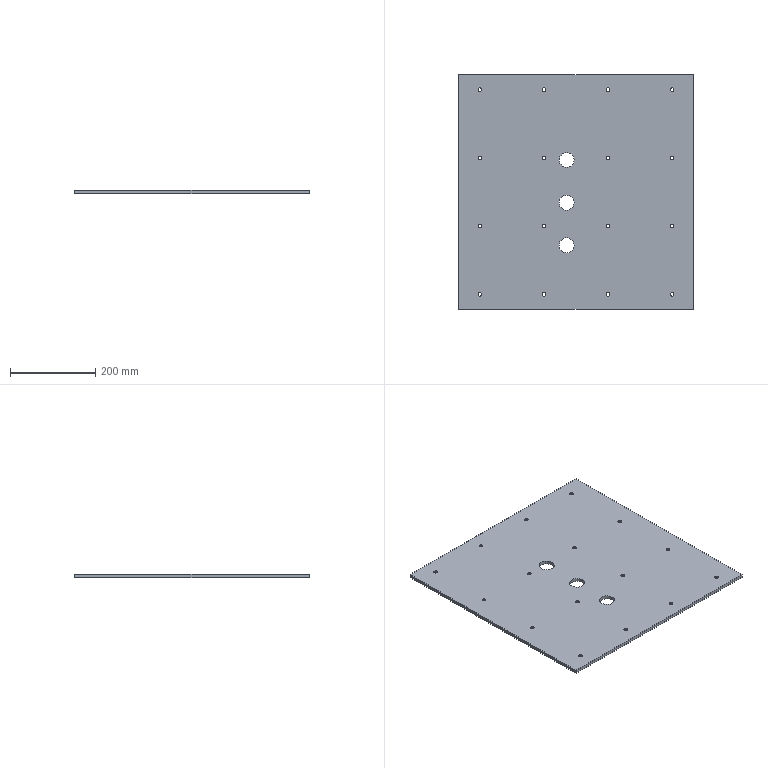Part | STEP file | 车灯-后视镜_id654_x_t | 1 solid | 57 faces | box 550 x 550 x 8 mm | volume 2381998 mm3 | cylinder 35 | cone 16 | plane 6 | commonest cylinder face diameters 8.5 x16 16 x16 35 x3
STEP:
#1=CARTESIAN_POINT('',(275.,-275.,-420.5));
#2=VERTEX_POINT('',#1);
#3=CARTESIAN_POINT('',(-275.,-275.,-420.5));
#4=VERTEX_POINT('',#3);
#5=CARTESIAN_POINT('',(275.,-275.,-420.5));
#6=DIRECTION('',(-1.,0.,0.));
#7=VECTOR('',#6,1.);
#8=LINE('',#5,#7);
#9=EDGE_CURVE('',#2,#4,#8,.T.);
#10=ORIENTED_EDGE('',*,*,#9,.T.);
#11=CARTESIAN_POINT('',(-275.,-275.,-428.5));
#12=VERTEX_POINT('',#11);
#13=CARTESIAN_POINT('',(-275.,-275.,-428.5));
#14=DIRECTION('',(0.,0.,1.));
#15=VECTOR('',#14,1.);
#16=LINE('',#13,#15);
#17=EDGE_CURVE('',#12,#4,#16,.T.);
#18=ORIENTED_EDGE('',*,*,#17,.F.);
#19=CARTESIAN_POINT('',(275.,-275.,-428.5));
#20=VERTEX_POINT('',#19);
#21=CARTESIAN_POINT('',(275.,-275.,-428.5));
#22=DIRECTION('',(-1.,0.,0.));
#23=VECTOR('',#22,1.);
#24=LINE('',#21,#23);
#25=EDGE_CURVE('',#20,#12,#24,.T.);
#26=ORIENTED_EDGE('',*,*,#25,.F.);
#27=CARTESIAN_POINT('',(275.,-275.,-428.5));
#28=DIRECTION('',(0.,0.,1.));
#29=VECTOR('',#28,1.);
#30=LINE('',#27,#29);
#31=EDGE_CURVE('',#20,#2,#30,.T.);
#32=ORIENTED_EDGE('',*,*,#31,.T.);
#33=EDGE_LOOP('',(#10,#18,#26,#32));
#34=FACE_OUTER_BOUND('',#33,.T.);
#35=CARTESIAN_POINT('',(275.,-275.,-428.5));
#36=DIRECTION('',(0.,-1.,0.));
#37=DIRECTION('',(0.,0.,1.));
#38=AXIS2_PLACEMENT_3D('',#35,#36,#37);
#39=PLANE('',#38);
#40=ADVANCED_FACE('',(#34),#39,.T.);
#41=CARTESIAN_POINT('',(-275.,275.,-420.5));
#42=VERTEX_POINT('',#41);
#43=CARTESIAN_POINT('',(-275.,-275.,-420.5));
#44=DIRECTION('',(0.,1.,0.));
#45=VECTOR('',#44,1.);
#46=LINE('',#43,#45);
#47=EDGE_CURVE('',#4,#42,#46,.T.);
#48=ORIENTED_EDGE('',*,*,#47,.T.);
#49=CARTESIAN_POINT('',(-275.,275.,-428.5));
#50=VERTEX_POINT('',#49);
#51=CARTESIAN_POINT('',(-275.,275.,-428.5));
#52=DIRECTION('',(0.,0.,1.));
#53=VECTOR('',#52,1.);
#54=LINE('',#51,#53);
#55=EDGE_CURVE('',#50,#42,#54,.T.);
#56=ORIENTED_EDGE('',*,*,#55,.F.);
#57=CARTESIAN_POINT('',(-275.,-275.,-428.5));
#58=DIRECTION('',(0.,1.,0.));
#59=VECTOR('',#58,1.);
#60=LINE('',#57,#59);
#61=EDGE_CURVE('',#12,#50,#60,.T.);
#62=ORIENTED_EDGE('',*,*,#61,.F.);
#63=ORIENTED_EDGE('',*,*,#17,.T.);
#64=EDGE_LOOP('',(#48,#56,#62,#63));
#65=FACE_OUTER_BOUND('',#64,.T.);
#66=CARTESIAN_POINT('',(-275.,-275.,-428.5));
#67=DIRECTION('',(-1.,0.,0.));
#68=DIRECTION('',(0.,0.,-1.));
#69=AXIS2_PLACEMENT_3D('',#66,#67,#68);
#70=PLANE('',#69);
#71=ADVANCED_FACE('',(#65),#70,.T.);
#72=CARTESIAN_POINT('',(275.,275.,-420.5));
#73=VERTEX_POINT('',#72);
#74=CARTESIAN_POINT('',(-275.,275.,-420.5));
#75=DIRECTION('',(1.,0.,0.));
#76=VECTOR('',#75,1.);
#77=LINE('',#74,#76);
#78=EDGE_CURVE('',#42,#73,#77,.T.);
#79=ORIENTED_EDGE('',*,*,#78,.T.);
#80=CARTESIAN_POINT('',(275.,275.,-428.5));
#81=VERTEX_POINT('',#80);
#82=CARTESIAN_POINT('',(275.,275.,-428.5));
#83=DIRECTION('',(0.,0.,1.));
#84=VECTOR('',#83,1.);
#85=LINE('',#82,#84);
#86=EDGE_CURVE('',#81,#73,#85,.T.);
#87=ORIENTED_EDGE('',*,*,#86,.F.);
#88=CARTESIAN_POINT('',(-275.,275.,-428.5));
#89=DIRECTION('',(1.,0.,0.));
#90=VECTOR('',#89,1.);
#91=LINE('',#88,#90);
#92=EDGE_CURVE('',#50,#81,#91,.T.);
#93=ORIENTED_EDGE('',*,*,#92,.F.);
#94=ORIENTED_EDGE('',*,*,#55,.T.);
#95=EDGE_LOOP('',(#79,#87,#93,#94));
#96=FACE_OUTER_BOUND('',#95,.T.);
#97=CARTESIAN_POINT('',(-275.,275.,-428.5));
#98=DIRECTION('',(0.,1.,0.));
#99=DIRECTION('',(0.,0.,-1.));
#100=AXIS2_PLACEMENT_3D('',#97,#98,#99);
#101=PLANE('',#100);
#102=ADVANCED_FACE('',(#96),#101,.T.);
#103=CARTESIAN_POINT('',(275.,275.,-420.5));
#104=DIRECTION('',(0.,-1.,0.));
#105=VECTOR('',#104,1.);
#106=LINE('',#103,#105);
#107=EDGE_CURVE('',#73,#2,#106,.T.);
#108=ORIENTED_EDGE('',*,*,#107,.T.);
#109=ORIENTED_EDGE('',*,*,#31,.F.);
#110=CARTESIAN_POINT('',(275.,275.,-428.5));
#111=DIRECTION('',(0.,-1.,0.));
#112=VECTOR('',#111,1.);
#113=LINE('',#110,#112);
#114=EDGE_CURVE('',#81,#20,#113,.T.);
#115=ORIENTED_EDGE('',*,*,#114,.F.);
#116=ORIENTED_EDGE('',*,*,#86,.T.);
#117=EDGE_LOOP('',(#108,#109,#115,#116));
#118=FACE_OUTER_BOUND('',#117,.T.);
#119=CARTESIAN_POINT('',(275.,275.,-428.5));
#120=DIRECTION('',(1.,0.,0.));
#121=DIRECTION('',(0.,0.,1.));
#122=AXIS2_PLACEMENT_3D('',#119,#120,#121);
#123=PLANE('',#122);
#124=ADVANCED_FACE('',(#118),#123,.T.);
#125=CARTESIAN_POINT('',(-83.,-80.,-428.5));
#126=VERTEX_POINT('',#125);
#127=CARTESIAN_POINT('',(-75.,-80.,-428.5));
#128=DIRECTION('',(0.,0.,-1.));
#129=DIRECTION('',(-1.,0.,0.));
#130=AXIS2_PLACEMENT_3D('',#127,#128,#129);
#131=CIRCLE('',#130,8.);
#132=EDGE_CURVE('',#126,#126,#131,.T.);
#133=ORIENTED_EDGE('',*,*,#132,.F.);
#134=EDGE_LOOP('',(#133));
#135=FACE_BOUND('',#134,.T.);
#136=CARTESIAN_POINT('',(-4.5,-125.,-428.5));
#137=VERTEX_POINT('',#136);
#138=CARTESIAN_POINT('',(-22.,-125.,-428.5));
#139=DIRECTION('',(0.,0.,1.));
#140=DIRECTION('',(1.,0.,0.));
#141=AXIS2_PLACEMENT_3D('',#138,#139,#140);
#142=CIRCLE('',#141,17.5);
#143=EDGE_CURVE('',#137,#137,#142,.T.);
#144=ORIENTED_EDGE('',*,*,#143,.T.);
#145=EDGE_LOOP('',(#144));
#146=FACE_BOUND('',#145,.T.);
#147=CARTESIAN_POINT('',(-4.5,-25.,-428.5));
#148=VERTEX_POINT('',#147);
#149=CARTESIAN_POINT('',(-22.,-25.,-428.5));
#150=DIRECTION('',(0.,0.,1.));
#151=DIRECTION('',(1.,0.,0.));
#152=AXIS2_PLACEMENT_3D('',#149,#150,#151);
#153=CIRCLE('',#152,17.5);
#154=EDGE_CURVE('',#148,#148,#153,.T.);
#155=ORIENTED_EDGE('',*,*,#154,.T.);
#156=EDGE_LOOP('',(#155));
#157=FACE_BOUND('',#156,.T.);
#158=CARTESIAN_POINT('',(-4.5,75.,-428.5));
#159=VERTEX_POINT('',#158);
#160=CARTESIAN_POINT('',(-22.,75.,-428.5));
#161=DIRECTION('',(0.,0.,1.));
#162=DIRECTION('',(1.,0.,0.));
#163=AXIS2_PLACEMENT_3D('',#160,#161,#162);
#164=CIRCLE('',#163,17.5);
#165=EDGE_CURVE('',#159,#159,#164,.T.);
#166=ORIENTED_EDGE('',*,*,#165,.T.);
#167=EDGE_LOOP('',(#166));
#168=FACE_BOUND('',#167,.T.);
#169=CARTESIAN_POINT('',(-233.,240.,-428.5));
#170=VERTEX_POINT('',#169);
#171=CARTESIAN_POINT('',(-225.,240.,-428.5));
#172=DIRECTION('',(0.,0.,-1.));
#173=DIRECTION('',(-1.,0.,0.));
#174=AXIS2_PLACEMENT_3D('',#171,#172,#173);
#175=CIRCLE('',#174,8.);
#176=EDGE_CURVE('',#170,#170,#175,.T.);
#177=ORIENTED_EDGE('',*,*,#176,.F.);
#178=EDGE_LOOP('',(#177));
#179=FACE_BOUND('',#178,.T.);
#180=CARTESIAN_POINT('',(-233.,-240.,-428.5));
#181=VERTEX_POINT('',#180);
#182=CARTESIAN_POINT('',(-225.,-240.,-428.5));
#183=DIRECTION('',(0.,0.,-1.));
#184=DIRECTION('',(-1.,0.,0.));
#185=AXIS2_PLACEMENT_3D('',#182,#183,#184);
#186=CIRCLE('',#185,8.);
#187=EDGE_CURVE('',#181,#181,#186,.T.);
#188=ORIENTED_EDGE('',*,*,#187,.F.);
#189=EDGE_LOOP('',(#188));
#190=FACE_BOUND('',#189,.T.);
#191=CARTESIAN_POINT('',(-83.,80.,-428.5));
#192=VERTEX_POINT('',#191);
#193=CARTESIAN_POINT('',(-75.,80.,-428.5));
#194=DIRECTION('',(0.,0.,-1.));
#195=DIRECTION('',(-1.,0.,0.));
#196=AXIS2_PLACEMENT_3D('',#193,#194,#195);
#197=CIRCLE('',#196,8.);
#198=EDGE_CURVE('',#192,#192,#197,.T.);
#199=ORIENTED_EDGE('',*,*,#198,.F.);
#200=EDGE_LOOP('',(#199));
#201=FACE_BOUND('',#200,.T.);
#202=CARTESIAN_POINT('',(-233.,-80.,-428.5));
#203=VERTEX_POINT('',#202);
#204=CARTESIAN_POINT('',(-225.,-80.,-428.5));
#205=DIRECTION('',(0.,0.,-1.));
#206=DIRECTION('',(-1.,0.,0.));
#207=AXIS2_PLACEMENT_3D('',#204,#205,#206);
#208=CIRCLE('',#207,8.);
#209=EDGE_CURVE('',#203,#203,#208,.T.);
#210=ORIENTED_EDGE('',*,*,#209,.F.);
#211=EDGE_LOOP('',(#210));
#212=FACE_BOUND('',#211,.T.);
#213=CARTESIAN_POINT('',(-233.,80.,-428.5));
#214=VERTEX_POINT('',#213);
#215=CARTESIAN_POINT('',(-225.,80.,-428.5));
#216=DIRECTION('',(0.,0.,-1.));
#217=DIRECTION('',(-1.,0.,0.));
#218=AXIS2_PLACEMENT_3D('',#215,#216,#217);
#219=CIRCLE('',#218,8.);
#220=EDGE_CURVE('',#214,#214,#219,.T.);
#221=ORIENTED_EDGE('',*,*,#220,.F.);
#222=EDGE_LOOP('',(#221));
#223=FACE_BOUND('',#222,.T.);
#224=CARTESIAN_POINT('',(-83.,-240.,-428.5));
#225=VERTEX_POINT('',#224);
#226=CARTESIAN_POINT('',(-75.,-240.,-428.5));
#227=DIRECTION('',(0.,0.,-1.));
#228=DIRECTION('',(-1.,0.,0.));
#229=AXIS2_PLACEMENT_3D('',#226,#227,#228);
#230=CIRCLE('',#229,8.);
#231=EDGE_CURVE('',#225,#225,#230,.T.);
#232=ORIENTED_EDGE('',*,*,#231,.F.);
#233=EDGE_LOOP('',(#232));
#234=FACE_BOUND('',#233,.T.);
#235=CARTESIAN_POINT('',(-83.,240.,-428.5));
#236=VERTEX_POINT('',#235);
#237=CARTESIAN_POINT('',(-75.,240.,-428.5));
#238=DIRECTION('',(0.,0.,-1.));
#239=DIRECTION('',(-1.,0.,0.));
#240=AXIS2_PLACEMENT_3D('',#237,#238,#239);
#241=CIRCLE('',#240,8.);
#242=EDGE_CURVE('',#236,#236,#241,.T.);
#243=ORIENTED_EDGE('',*,*,#242,.F.);
#244=EDGE_LOOP('',(#243));
#245=FACE_BOUND('',#244,.T.);
#246=CARTESIAN_POINT('',(67.,240.,-428.5));
#247=VERTEX_POINT('',#246);
#248=CARTESIAN_POINT('',(75.,240.,-428.5));
#249=DIRECTION('',(0.,0.,-1.));
#250=DIRECTION('',(-1.,0.,0.));
#251=AXIS2_PLACEMENT_3D('',#248,#249,#250);
#252=CIRCLE('',#251,8.);
#253=EDGE_CURVE('',#247,#247,#252,.T.);
#254=ORIENTED_EDGE('',*,*,#253,.F.);
#255=EDGE_LOOP('',(#254));
#256=FACE_BOUND('',#255,.T.);
#257=CARTESIAN_POINT('',(217.,80.,-428.5));
#258=VERTEX_POINT('',#257);
#259=CARTESIAN_POINT('',(225.,80.,-428.5));
#260=DIRECTION('',(0.,0.,-1.));
#261=DIRECTION('',(-1.,0.,0.));
#262=AXIS2_PLACEMENT_3D('',#259,#260,#261);
#263=CIRCLE('',#262,8.);
#264=EDGE_CURVE('',#258,#258,#263,.T.);
#265=ORIENTED_EDGE('',*,*,#264,.F.);
#266=EDGE_LOOP('',(#265));
#267=FACE_BOUND('',#266,.T.);
#268=CARTESIAN_POINT('',(217.,240.,-428.5));
#269=VERTEX_POINT('',#268);
#270=CARTESIAN_POINT('',(225.,240.,-428.5));
#271=DIRECTION('',(0.,0.,-1.));
#272=DIRECTION('',(-1.,0.,0.));
#273=AXIS2_PLACEMENT_3D('',#270,#271,#272);
#274=CIRCLE('',#273,8.);
#275=EDGE_CURVE('',#269,#269,#274,.T.);
#276=ORIENTED_EDGE('',*,*,#275,.F.);
#277=EDGE_LOOP('',(#276));
#278=FACE_BOUND('',#277,.T.);
#279=CARTESIAN_POINT('',(67.,-240.,-428.5));
#280=VERTEX_POINT('',#279);
#281=CARTESIAN_POINT('',(75.,-240.,-428.5));
#282=DIRECTION('',(0.,0.,-1.));
#283=DIRECTION('',(-1.,0.,0.));
#284=AXIS2_PLACEMENT_3D('',#281,#282,#283);
#285=CIRCLE('',#284,8.);
#286=EDGE_CURVE('',#280,#280,#285,.T.);
#287=ORIENTED_EDGE('',*,*,#286,.F.);
#288=EDGE_LOOP('',(#287));
#289=FACE_BOUND('',#288,.T.);
#290=CARTESIAN_POINT('',(217.,-240.,-428.5));
#291=VERTEX_POINT('',#290);
#292=CARTESIAN_POINT('',(225.,-240.,-428.5));
#293=DIRECTION('',(0.,0.,-1.));
#294=DIRECTION('',(-1.,0.,0.));
#295=AXIS2_PLACEMENT_3D('',#292,#293,#294);
#296=CIRCLE('',#295,8.);
#297=EDGE_CURVE('',#291,#291,#296,.T.);
#298=ORIENTED_EDGE('',*,*,#297,.F.);
#299=EDGE_LOOP('',(#298));
#300=FACE_BOUND('',#299,.T.);
#301=CARTESIAN_POINT('',(67.,-80.,-428.5));
#302=VERTEX_POINT('',#301);
#303=CARTESIAN_POINT('',(75.,-80.,-428.5));
#304=DIRECTION('',(0.,0.,-1.));
#305=DIRECTION('',(-1.,0.,0.));
#306=AXIS2_PLACEMENT_3D('',#303,#304,#305);
#307=CIRCLE('',#306,8.);
#308=EDGE_CURVE('',#302,#302,#307,.T.);
#309=ORIENTED_EDGE('',*,*,#308,.F.);
#310=EDGE_LOOP('',(#309));
#311=FACE_BOUND('',#310,.T.);
#312=CARTESIAN_POINT('',(217.,-80.,-428.5));
#313=VERTEX_POINT('',#312);
#314=CARTESIAN_POINT('',(225.,-80.,-428.5));
#315=DIRECTION('',(0.,0.,-1.));
#316=DIRECTION('',(-1.,0.,0.));
#317=AXIS2_PLACEMENT_3D('',#314,#315,#316);
#318=CIRCLE('',#317,8.);
#319=EDGE_CURVE('',#313,#313,#318,.T.);
#320=ORIENTED_EDGE('',*,*,#319,.F.);
#321=EDGE_LOOP('',(#320));
#322=FACE_BOUND('',#321,.T.);
#323=CARTESIAN_POINT('',(67.,80.,-428.5));
#324=VERTEX_POINT('',#323);
#325=CARTESIAN_POINT('',(75.,80.,-428.5));
#326=DIRECTION('',(0.,0.,-1.));
#327=DIRECTION('',(-1.,0.,0.));
#328=AXIS2_PLACEMENT_3D('',#325,#326,#327);
#329=CIRCLE('',#328,8.);
#330=EDGE_CURVE('',#324,#324,#329,.T.);
#331=ORIENTED_EDGE('',*,*,#330,.F.);
#332=EDGE_LOOP('',(#331));
#333=FACE_BOUND('',#332,.T.);
#334=ORIENTED_EDGE('',*,*,#25,.T.);
#335=ORIENTED_EDGE('',*,*,#61,.T.);
#336=ORIENTED_EDGE('',*,*,#92,.T.);
#337=ORIENTED_EDGE('',*,*,#114,.T.);
#338=EDGE_LOOP('',(#334,#335,#336,#337));
#339=FACE_BOUND('',#338,.T.);
#340=CARTESIAN_POINT('',(-275.,-275.,-428.5));
#341=DIRECTION('',(0.,0.,1.));
#342=DIRECTION('',(-1.,0.,0.));
#343=AXIS2_PLACEMENT_3D('',#340,#341,#342);
#344=PLANE('',#343);
#345=ADVANCED_FACE('',(#135,#146,#157,#168,#179,#190,#201,#212,#223,#234,#245,#256,#267,#278,#289,#300,#311,#322,#333,#339),#344,.F.);
#346=CARTESIAN_POINT('',(-79.25,-80.,-420.5));
#347=VERTEX_POINT('',#346);
#348=CARTESIAN_POINT('',(-75.,-80.,-420.5));
#349=DIRECTION('',(0.,0.,-1.));
#350=DIRECTION('',(-1.,0.,0.));
#351=AXIS2_PLACEMENT_3D('',#348,#349,#350);
#352=CIRCLE('',#351,4.25);
#353=EDGE_CURVE('',#347,#347,#352,.T.);
#354=ORIENTED_EDGE('',*,*,#353,.T.);
#355=EDGE_LOOP('',(#354));
#356=FACE_BOUND('',#355,.T.);
#357=CARTESIAN_POINT('',(-4.5,-125.,-420.5));
#358=VERTEX_POINT('',#357);
#359=CARTESIAN_POINT('',(-22.,-125.,-420.5));
#360=DIRECTION('',(0.,0.,1.));
#361=DIRECTION('',(1.,0.,0.));
#362=AXIS2_PLACEMENT_3D('',#359,#360,#361);
#363=CIRCLE('',#362,17.5);
#364=EDGE_CURVE('',#358,#358,#363,.T.);
#365=ORIENTED_EDGE('',*,*,#364,.F.);
#366=EDGE_LOOP('',(#365));
#367=FACE_BOUND('',#366,.T.);
#368=CARTESIAN_POINT('',(-4.5,-25.,-420.5));
#369=VERTEX_POINT('',#368);
#370=CARTESIAN_POINT('',(-22.,-25.,-420.5));
#371=DIRECTION('',(0.,0.,1.));
#372=DIRECTION('',(1.,0.,0.));
#373=AXIS2_PLACEMENT_3D('',#370,#371,#372);
#374=CIRCLE('',#373,17.5);
#375=EDGE_CURVE('',#369,#369,#374,.T.);
#376=ORIENTED_EDGE('',*,*,#375,.F.);
#377=EDGE_LOOP('',(#376));
#378=FACE_BOUND('',#377,.T.);
#379=CARTESIAN_POINT('',(-4.5,75.,-420.5));
#380=VERTEX_POINT('',#379);
#381=CARTESIAN_POINT('',(-22.,75.,-420.5));
#382=DIRECTION('',(0.,0.,1.));
#383=DIRECTION('',(1.,0.,0.));
#384=AXIS2_PLACEMENT_3D('',#381,#382,#383);
#385=CIRCLE('',#384,17.5);
#386=EDGE_CURVE('',#380,#380,#385,.T.);
#387=ORIENTED_EDGE('',*,*,#386,.F.);
#388=EDGE_LOOP('',(#387));
#389=FACE_BOUND('',#388,.T.);
#390=CARTESIAN_POINT('',(-229.25,240.,-420.5));
#391=VERTEX_POINT('',#390);
#392=CARTESIAN_POINT('',(-225.,240.,-420.5));
#393=DIRECTION('',(0.,0.,-1.));
#394=DIRECTION('',(-1.,0.,0.));
#395=AXIS2_PLACEMENT_3D('',#392,#393,#394);
#396=CIRCLE('',#395,4.25);
#397=EDGE_CURVE('',#391,#391,#396,.T.);
#398=ORIENTED_EDGE('',*,*,#397,.T.);
#399=EDGE_LOOP('',(#398));
#400=FACE_BOUND('',#399,.T.);
#401=CARTESIAN_POINT('',(-229.25,-240.,-420.5));
#402=VERTEX_POINT('',#401);
#403=CARTESIAN_POINT('',(-225.,-240.,-420.5));
#404=DIRECTION('',(0.,0.,-1.));
#405=DIRECTION('',(-1.,0.,0.));
#406=AXIS2_PLACEMENT_3D('',#403,#404,#405);
#407=CIRCLE('',#406,4.25);
#408=EDGE_CURVE('',#402,#402,#407,.T.);
#409=ORIENTED_EDGE('',*,*,#408,.T.);
#410=EDGE_LOOP('',(#409));
#411=FACE_BOUND('',#410,.T.);
#412=CARTESIAN_POINT('',(-79.25,80.,-420.5));
#413=VERTEX_POINT('',#412);
#414=CARTESIAN_POINT('',(-75.,80.,-420.5));
#415=DIRECTION('',(0.,0.,-1.));
#416=DIRECTION('',(-1.,0.,0.));
#417=AXIS2_PLACEMENT_3D('',#414,#415,#416);
#418=CIRCLE('',#417,4.25);
#419=EDGE_CURVE('',#413,#413,#418,.T.);
#420=ORIENTED_EDGE('',*,*,#419,.T.);
#421=EDGE_LOOP('',(#420));
#422=FACE_BOUND('',#421,.T.);
#423=CARTESIAN_POINT('',(-229.25,-80.,-420.5));
#424=VERTEX_POINT('',#423);
#425=CARTESIAN_POINT('',(-225.,-80.,-420.5));
#426=DIRECTION('',(0.,0.,-1.));
#427=DIRECTION('',(-1.,0.,0.));
#428=AXIS2_PLACEMENT_3D('',#425,#426,#427);
#429=CIRCLE('',#428,4.25);
#430=EDGE_CURVE('',#424,#424,#429,.T.);
#431=ORIENTED_EDGE('',*,*,#430,.T.);
#432=EDGE_LOOP('',(#431));
#433=FACE_BOUND('',#432,.T.);
#434=CARTESIAN_POINT('',(-229.25,80.,-420.5));
#435=VERTEX_POINT('',#434);
#436=CARTESIAN_POINT('',(-225.,80.,-420.5));
#437=DIRECTION('',(0.,0.,-1.));
#438=DIRECTION('',(-1.,0.,0.));
#439=AXIS2_PLACEMENT_3D('',#436,#437,#438);
#440=CIRCLE('',#439,4.25);
#441=EDGE_CURVE('',#435,#435,#440,.T.);
#442=ORIENTED_EDGE('',*,*,#441,.T.);
#443=EDGE_LOOP('',(#442));
#444=FACE_BOUND('',#443,.T.);
#445=CARTESIAN_POINT('',(-79.25,-240.,-420.5));
#446=VERTEX_POINT('',#445);
#447=CARTESIAN_POINT('',(-75.,-240.,-420.5));
#448=DIRECTION('',(0.,0.,-1.));
#449=DIRECTION('',(-1.,0.,0.));
#450=AXIS2_PLACEMENT_3D('',#447,#448,#449);
#451=CIRCLE('',#450,4.25);
#452=EDGE_CURVE('',#446,#446,#451,.T.);
#453=ORIENTED_EDGE('',*,*,#452,.T.);
#454=EDGE_LOOP('',(#453));
#455=FACE_BOUND('',#454,.T.);
#456=CARTESIAN_POINT('',(-79.25,240.,-420.5));
#457=VERTEX_POINT('',#456);
#458=CARTESIAN_POINT('',(-75.,240.,-420.5));
#459=DIRECTION('',(0.,0.,-1.));
#460=DIRECTION('',(-1.,0.,0.));
#461=AXIS2_PLACEMENT_3D('',#458,#459,#460);
#462=CIRCLE('',#461,4.25);
#463=EDGE_CURVE('',#457,#457,#462,.T.);
#464=ORIENTED_EDGE('',*,*,#463,.T.);
#465=EDGE_LOOP('',(#464));
#466=FACE_BOUND('',#465,.T.);
#467=CARTESIAN_POINT('',(70.75,240.,-420.5));
#468=VERTEX_POINT('',#467);
#469=CARTESIAN_POINT('',(75.,240.,-420.5));
#470=DIRECTION('',(0.,0.,-1.));
#471=DIRECTION('',(-1.,0.,0.));
#472=AXIS2_PLACEMENT_3D('',#469,#470,#471);
#473=CIRCLE('',#472,4.25);
#474=EDGE_CURVE('',#468,#468,#473,.T.);
#475=ORIENTED_EDGE('',*,*,#474,.T.);
#476=EDGE_LOOP('',(#475));
#477=FACE_BOUND('',#476,.T.);
#478=CARTESIAN_POINT('',(220.75,80.,-420.5));
#479=VERTEX_POINT('',#478);
#480=CARTESIAN_POINT('',(225.,80.,-420.5));
#481=DIRECTION('',(0.,0.,-1.));
#482=DIRECTION('',(-1.,0.,0.));
#483=AXIS2_PLACEMENT_3D('',#480,#481,#482);
#484=CIRCLE('',#483,4.25);
#485=EDGE_CURVE('',#479,#479,#484,.T.);
#486=ORIENTED_EDGE('',*,*,#485,.T.);
#487=EDGE_LOOP('',(#486));
#488=FACE_BOUND('',#487,.T.);
#489=CARTESIAN_POINT('',(220.75,240.,-420.5));
#490=VERTEX_POINT('',#489);
#491=CARTESIAN_POINT('',(225.,240.,-420.5));
#492=DIRECTION('',(0.,0.,-1.));
#493=DIRECTION('',(-1.,0.,0.));
#494=AXIS2_PLACEMENT_3D('',#491,#492,#493);
#495=CIRCLE('',#494,4.25);
#496=EDGE_CURVE('',#490,#490,#495,.T.);
#497=ORIENTED_EDGE('',*,*,#496,.T.);
#498=EDGE_LOOP('',(#497));
#499=FACE_BOUND('',#498,.T.);
#500=CARTESIAN_POINT('',(70.75,-240.,-420.5));
#501=VERTEX_POINT('',#500);
#502=CARTESIAN_POINT('',(75.,-240.,-420.5));
#503=DIRECTION('',(0.,0.,-1.));
#504=DIRECTION('',(-1.,0.,0.));
#505=AXIS2_PLACEMENT_3D('',#502,#503,#504);
#506=CIRCLE('',#505,4.25);
#507=EDGE_CURVE('',#501,#501,#506,.T.);
#508=ORIENTED_EDGE('',*,*,#507,.T.);
#509=EDGE_LOOP('',(#508));
#510=FACE_BOUND('',#509,.T.);
#511=CARTESIAN_POINT('',(220.75,-240.,-420.5));
#512=VERTEX_POINT('',#511);
#513=CARTESIAN_POINT('',(225.,-240.,-420.5));
#514=DIRECTION('',(0.,0.,-1.));
#515=DIRECTION('',(-1.,0.,0.));
#516=AXIS2_PLACEMENT_3D('',#513,#514,#515);
#517=CIRCLE('',#516,4.25);
#518=EDGE_CURVE('',#512,#512,#517,.T.);
#519=ORIENTED_EDGE('',*,*,#518,.T.);
#520=EDGE_LOOP('',(#519));
#521=FACE_BOUND('',#520,.T.);
#522=CARTESIAN_POINT('',(70.75,-80.,-420.5));
#523=VERTEX_POINT('',#522);
#524=CARTESIAN_POINT('',(75.,-80.,-420.5));
#525=DIRECTION('',(0.,0.,-1.));
#526=DIRECTION('',(-1.,0.,0.));
#527=AXIS2_PLACEMENT_3D('',#524,#525,#526);
#528=CIRCLE('',#527,4.25);
#529=EDGE_CURVE('',#523,#523,#528,.T.);
#530=ORIENTED_EDGE('',*,*,#529,.T.);
#531=EDGE_LOOP('',(#530));
#532=FACE_BOUND('',#531,.T.);
#533=CARTESIAN_POINT('',(220.75,-80.,-420.5));
#534=VERTEX_POINT('',#533);
#535=CARTESIAN_POINT('',(225.,-80.,-420.5));
#536=DIRECTION('',(0.,0.,-1.));
#537=DIRECTION('',(-1.,0.,0.));
#538=AXIS2_PLACEMENT_3D('',#535,#536,#537);
#539=CIRCLE('',#538,4.25);
#540=EDGE_CURVE('',#534,#534,#539,.T.);
#541=ORIENTED_EDGE('',*,*,#540,.T.);
#542=EDGE_LOOP('',(#541));
#543=FACE_BOUND('',#542,.T.);
#544=CARTESIAN_POINT('',(70.75,80.,-420.5));
#545=VERTEX_POINT('',#544);
#546=CARTESIAN_POINT('',(75.,80.,-420.5));
#547=DIRECTION('',(0.,0.,-1.));
#548=DIRECTION('',(-1.,0.,0.));
#549=AXIS2_PLACEMENT_3D('',#546,#547,#548);
#550=CIRCLE('',#549,4.25);
#551=EDGE_CURVE('',#545,#545,#550,.T.);
#552=ORIENTED_EDGE('',*,*,#551,.T.);
#553=EDGE_LOOP('',(#552));
#554=FACE_BOUND('',#553,.T.);
#555=ORIENTED_EDGE('',*,*,#9,.F.);
#556=ORIENTED_EDGE('',*,*,#107,.F.);
#557=ORIENTED_EDGE('',*,*,#78,.F.);
#558=ORIENTED_EDGE('',*,*,#47,.F.);
#559=EDGE_LOOP('',(#555,#556,#557,#558));
#560=FACE_BOUND('',#559,.T.);
#561=CARTESIAN_POINT('',(-275.,-275.,-420.5));
#562=DIRECTION('',(0.,0.,1.));
#563=DIRECTION('',(-1.,0.,0.));
#564=AXIS2_PLACEMENT_3D('',#561,#562,#563);
#565=PLANE('',#564);
#566=ADVANCED_FACE('',(#356,#367,#378,#389,#400,#411,#422,#433,#444,#455,#466,#477,#488,#499,#510,#521,#532,#543,#554,#560),#565,.T.);
#567=ORIENTED_EDGE('',*,*,#551,.F.);
#568=EDGE_LOOP('',(#567));
#569=FACE_BOUND('',#568,.T.);
#570=CARTESIAN_POINT('',(70.75,80.,-423.122));
#571=VERTEX_POINT('',#570);
#572=CARTESIAN_POINT('',(75.,80.,-423.122));
#573=DIRECTION('',(0.,0.,-1.));
#574=DIRECTION('',(-1.,0.,0.));
#575=AXIS2_PLACEMENT_3D('',#572,#573,#574);
#576=CIRCLE('',#575,4.25);
#577=EDGE_CURVE('',#571,#571,#576,.T.);
#578=ORIENTED_EDGE('',*,*,#577,.T.);
#579=EDGE_LOOP('',(#578));
#580=FACE_BOUND('',#579,.T.);
#581=CARTESIAN_POINT('',(75.,80.,-423.6));
#582=DIRECTION('',(0.,0.,1.));
#583=DIRECTION('',(1.,0.,0.));
#584=AXIS2_PLACEMENT_3D('',#581,#582,#583);
#585=CYLINDRICAL_SURFACE('',#584,4.25);
#586=ADVANCED_FACE('',(#569,#580),#585,.F.);
#587=CARTESIAN_POINT('',(67.,80.,-426.872));
#588=VERTEX_POINT('',#587);
#589=CARTESIAN_POINT('',(75.,80.,-426.872));
#590=DIRECTION('',(0.,0.,-1.));
#591=DIRECTION('',(-1.,0.,0.));
#592=AXIS2_PLACEMENT_3D('',#589,#590,#591);
#593=CIRCLE('',#592,8.);
#594=EDGE_CURVE('',#588,#588,#593,.T.);
#595=ORIENTED_EDGE('',*,*,#594,.F.);
#596=EDGE_LOOP('',(#595));
#597=FACE_BOUND('',#596,.T.);
#598=ORIENTED_EDGE('',*,*,#330,.T.);
#599=EDGE_LOOP('',(#598));
#600=FACE_BOUND('',#599,.T.);
#601=CARTESIAN_POINT('',(75.,80.,-428.));
#602=DIRECTION('',(0.,0.,1.));
#603=DIRECTION('',(1.,0.,0.));
#604=AXIS2_PLACEMENT_3D('',#601,#602,#603);
#605=CYLINDRICAL_SURFACE('',#604,8.);
#606=ADVANCED_FACE('',(#597,#600),#605,.F.);
#607=ORIENTED_EDGE('',*,*,#577,.F.);
#608=EDGE_LOOP('',(#607));
#609=FACE_BOUND('',#608,.T.);
#610=ORIENTED_EDGE('',*,*,#594,.T.);
#611=EDGE_LOOP('',(#610));
#612=FACE_BOUND('',#611,.T.);
#613=CARTESIAN_POINT('',(75.,80.,-426.286));
#614=DIRECTION('',(0.,0.,-1.));
#615=DIRECTION('',(1.,0.,0.));
#616=AXIS2_PLACEMENT_3D('',#613,#614,#615);
#617=CONICAL_SURFACE('',#616,7.414,45.);
#618=ADVANCED_FACE('',(#609,#612),#617,.F.);
#619=ORIENTED_EDGE('',*,*,#540,.F.);
#620=EDGE_LOOP('',(#619));
#621=FACE_BOUND('',#620,.T.);
#622=CARTESIAN_POINT('',(220.75,-80.,-423.122));
#623=VERTEX_POINT('',#622);
#624=CARTESIAN_POINT('',(225.,-80.,-423.122));
#625=DIRECTION('',(0.,0.,-1.));
#626=DIRECTION('',(-1.,0.,0.));
#627=AXIS2_PLACEMENT_3D('',#624,#625,#626);
#628=CIRCLE('',#627,4.25);
#629=EDGE_CURVE('',#623,#623,#628,.T.);
#630=ORIENTED_EDGE('',*,*,#629,.T.);
#631=EDGE_LOOP('',(#630));
#632=FACE_BOUND('',#631,.T.);
#633=CARTESIAN_POINT('',(225.,-80.,-423.6));
#634=DIRECTION('',(0.,0.,1.));
#635=DIRECTION('',(1.,0.,0.));
#636=AXIS2_PLACEMENT_3D('',#633,#634,#635);
#637=CYLINDRICAL_SURFACE('',#636,4.25);
#638=ADVANCED_FACE('',(#621,#632),#637,.F.);
#639=CARTESIAN_POINT('',(217.,-80.,-426.872));
#640=VERTEX_POINT('',#639);
#641=CARTESIAN_POINT('',(225.,-80.,-426.872));
#642=DIRECTION('',(0.,0.,-1.));
#643=DIRECTION('',(-1.,0.,0.));
#644=AXIS2_PLACEMENT_3D('',#641,#642,#643);
#645=CIRCLE('',#644,8.);
#646=EDGE_CURVE('',#640,#640,#645,.T.);
#647=ORIENTED_EDGE('',*,*,#646,.F.);
#648=EDGE_LOOP('',(#647));
#649=FACE_BOUND('',#648,.T.);
#650=ORIENTED_EDGE('',*,*,#319,.T.);
#651=EDGE_LOOP('',(#650));
#652=FACE_BOUND('',#651,.T.);
#653=CARTESIAN_POINT('',(225.,-80.,-428.));
#654=DIRECTION('',(0.,0.,1.));
#655=DIRECTION('',(1.,0.,0.));
#656=AXIS2_PLACEMENT_3D('',#653,#654,#655);
#657=CYLINDRICAL_SURFACE('',#656,8.);
#658=ADVANCED_FACE('',(#649,#652),#657,.F.);
#659=ORIENTED_EDGE('',*,*,#629,.F.);
#660=EDGE_LOOP('',(#659));
#661=FACE_BOUND('',#660,.T.);
#662=ORIENTED_EDGE('',*,*,#646,.T.);
#663=EDGE_LOOP('',(#662));
#664=FACE_BOUND('',#663,.T.);
#665=CARTESIAN_POINT('',(225.,-80.,-426.286));
#666=DIRECTION('',(0.,0.,-1.));
#667=DIRECTION('',(1.,0.,0.));
#668=AXIS2_PLACEMENT_3D('',#665,#666,#667);
#669=CONICAL_SURFACE('',#668,7.414,45.);
#670=ADVANCED_FACE('',(#661,#664),#669,.F.);
#671=ORIENTED_EDGE('',*,*,#529,.F.);
#672=EDGE_LOOP('',(#671));
#673=FACE_BOUND('',#672,.T.);
#674=CARTESIAN_POINT('',(70.75,-80.,-423.122));
#675=VERTEX_POINT('',#674);
#676=CARTESIAN_POINT('',(75.,-80.,-423.122));
#677=DIRECTION('',(0.,0.,-1.));
#678=DIRECTION('',(-1.,0.,0.));
#679=AXIS2_PLACEMENT_3D('',#676,#677,#678);
#680=CIRCLE('',#679,4.25);
#681=EDGE_CURVE('',#675,#675,#680,.T.);
#682=ORIENTED_EDGE('',*,*,#681,.T.);
#683=EDGE_LOOP('',(#682));
#684=FACE_BOUND('',#683,.T.);
#685=CARTESIAN_POINT('',(75.,-80.,-423.6));
#686=DIRECTION('',(0.,0.,1.));
#687=DIRECTION('',(1.,0.,0.));
#688=AXIS2_PLACEMENT_3D('',#685,#686,#687);
#689=CYLINDRICAL_SURFACE('',#688,4.25);
#690=ADVANCED_FACE('',(#673,#684),#689,.F.);
#691=CARTESIAN_POINT('',(67.,-80.,-426.872));
#692=VERTEX_POINT('',#691);
#693=CARTESIAN_POINT('',(75.,-80.,-426.872));
#694=DIRECTION('',(0.,0.,-1.));
#695=DIRECTION('',(-1.,0.,0.));
#696=AXIS2_PLACEMENT_3D('',#693,#694,#695);
#697=CIRCLE('',#696,8.);
#698=EDGE_CURVE('',#692,#692,#697,.T.);
#699=ORIENTED_EDGE('',*,*,#698,.F.);
#700=EDGE_LOOP('',(#699));
#701=FACE_BOUND('',#700,.T.);
#702=ORIENTED_EDGE('',*,*,#308,.T.);
#703=EDGE_LOOP('',(#702));
#704=FACE_BOUND('',#703,.T.);
#705=CARTESIAN_POINT('',(75.,-80.,-428.));
#706=DIRECTION('',(0.,0.,1.));
#707=DIRECTION('',(1.,0.,0.));
#708=AXIS2_PLACEMENT_3D('',#705,#706,#707);
#709=CYLINDRICAL_SURFACE('',#708,8.);
#710=ADVANCED_FACE('',(#701,#704),#709,.F.);
#711=ORIENTED_EDGE('',*,*,#681,.F.);
#712=EDGE_LOOP('',(#711));
#713=FACE_BOUND('',#712,.T.);
#714=ORIENTED_EDGE('',*,*,#698,.T.);
#715=EDGE_LOOP('',(#714));
#716=FACE_BOUND('',#715,.T.);
#717=CARTESIAN_POINT('',(75.,-80.,-426.286));
#718=DIRECTION('',(0.,0.,-1.));
#719=DIRECTION('',(1.,0.,0.));
#720=AXIS2_PLACEMENT_3D('',#717,#718,#719);
#721=CONICAL_SURFACE('',#720,7.414,45.);
#722=ADVANCED_FACE('',(#713,#716),#721,.F.);
#723=ORIENTED_EDGE('',*,*,#518,.F.);
#724=EDGE_LOOP('',(#723));
#725=FACE_BOUND('',#724,.T.);
#726=CARTESIAN_POINT('',(220.75,-240.,-423.122));
#727=VERTEX_POINT('',#726);
#728=CARTESIAN_POINT('',(225.,-240.,-423.122));
#729=DIRECTION('',(0.,0.,-1.));
#730=DIRECTION('',(-1.,0.,0.));
#731=AXIS2_PLACEMENT_3D('',#728,#729,#730);
#732=CIRCLE('',#731,4.25);
#733=EDGE_CURVE('',#727,#727,#732,.T.);
#734=ORIENTED_EDGE('',*,*,#733,.T.);
#735=EDGE_LOOP('',(#734));
#736=FACE_BOUND('',#735,.T.);
#737=CARTESIAN_POINT('',(225.,-240.,-423.6));
#738=DIRECTION('',(0.,0.,1.));
#739=DIRECTION('',(1.,0.,0.));
#740=AXIS2_PLACEMENT_3D('',#737,#738,#739);
#741=CYLINDRICAL_SURFACE('',#740,4.25);
#742=ADVANCED_FACE('',(#725,#736),#741,.F.);
#743=CARTESIAN_POINT('',(217.,-240.,-426.872));
#744=VERTEX_POINT('',#743);
#745=CARTESIAN_POINT('',(225.,-240.,-426.872));
#746=DIRECTION('',(0.,0.,-1.));
#747=DIRECTION('',(-1.,0.,0.));
#748=AXIS2_PLACEMENT_3D('',#745,#746,#747);
#749=CIRCLE('',#748,8.);
#750=EDGE_CURVE('',#744,#744,#749,.T.);
#751=ORIENTED_EDGE('',*,*,#750,.F.);
#752=EDGE_LOOP('',(#751));
#753=FACE_BOUND('',#752,.T.);
#754=ORIENTED_EDGE('',*,*,#297,.T.);
#755=EDGE_LOOP('',(#754));
#756=FACE_BOUND('',#755,.T.);
#757=CARTESIAN_POINT('',(225.,-240.,-428.));
#758=DIRECTION('',(0.,0.,1.));
#759=DIRECTION('',(1.,0.,0.));
#760=AXIS2_PLACEMENT_3D('',#757,#758,#759);
#761=CYLINDRICAL_SURFACE('',#760,8.);
#762=ADVANCED_FACE('',(#753,#756),#761,.F.);
#763=ORIENTED_EDGE('',*,*,#733,.F.);
#764=EDGE_LOOP('',(#763));
#765=FACE_BOUND('',#764,.T.);
#766=ORIENTED_EDGE('',*,*,#750,.T.);
#767=EDGE_LOOP('',(#766));
#768=FACE_BOUND('',#767,.T.);
#769=CARTESIAN_POINT('',(225.,-240.,-426.286));
#770=DIRECTION('',(0.,0.,-1.));
#771=DIRECTION('',(1.,0.,0.));
#772=AXIS2_PLACEMENT_3D('',#769,#770,#771);
#773=CONICAL_SURFACE('',#772,7.414,45.);
#774=ADVANCED_FACE('',(#765,#768),#773,.F.);
#775=ORIENTED_EDGE('',*,*,#507,.F.);
#776=EDGE_LOOP('',(#775));
#777=FACE_BOUND('',#776,.T.);
#778=CARTESIAN_POINT('',(70.75,-240.,-423.122));
#779=VERTEX_POINT('',#778);
#780=CARTESIAN_POINT('',(75.,-240.,-423.122));
#781=DIRECTION('',(0.,0.,-1.));
#782=DIRECTION('',(-1.,0.,0.));
#783=AXIS2_PLACEMENT_3D('',#780,#781,#782);
#784=CIRCLE('',#783,4.25);
#785=EDGE_CURVE('',#779,#779,#784,.T.);
#786=ORIENTED_EDGE('',*,*,#785,.T.);
#787=EDGE_LOOP('',(#786));
#788=FACE_BOUND('',#787,.T.);
#789=CARTESIAN_POINT('',(75.,-240.,-423.6));
#790=DIRECTION('',(0.,0.,1.));
#791=DIRECTION('',(1.,0.,0.));
#792=AXIS2_PLACEMENT_3D('',#789,#790,#791);
#793=CYLINDRICAL_SURFACE('',#792,4.25);
#794=ADVANCED_FACE('',(#777,#788),#793,.F.);
#795=CARTESIAN_POINT('',(67.,-240.,-426.872));
#796=VERTEX_POINT('',#795);
#797=CARTESIAN_POINT('',(75.,-240.,-426.872));
#798=DIRECTION('',(0.,0.,-1.));
#799=DIRECTION('',(-1.,0.,0.));
#800=AXIS2_PLACEMENT_3D('',#797,#798,#799);
#801=CIRCLE('',#800,8.);
#802=EDGE_CURVE('',#796,#796,#801,.T.);
#803=ORIENTED_EDGE('',*,*,#802,.F.);
#804=EDGE_LOOP('',(#803));
#805=FACE_BOUND('',#804,.T.);
#806=ORIENTED_EDGE('',*,*,#286,.T.);
#807=EDGE_LOOP('',(#806));
#808=FACE_BOUND('',#807,.T.);
#809=CARTESIAN_POINT('',(75.,-240.,-428.));
#810=DIRECTION('',(0.,0.,1.));
#811=DIRECTION('',(1.,0.,0.));
#812=AXIS2_PLACEMENT_3D('',#809,#810,#811);
#813=CYLINDRICAL_SURFACE('',#812,8.);
#814=ADVANCED_FACE('',(#805,#808),#813,.F.);
#815=ORIENTED_EDGE('',*,*,#785,.F.);
#816=EDGE_LOOP('',(#815));
#817=FACE_BOUND('',#816,.T.);
#818=ORIENTED_EDGE('',*,*,#802,.T.);
#819=EDGE_LOOP('',(#818));
#820=FACE_BOUND('',#819,.T.);
#821=CARTESIAN_POINT('',(75.,-240.,-426.286));
#822=DIRECTION('',(0.,0.,-1.));
#823=DIRECTION('',(1.,0.,0.));
#824=AXIS2_PLACEMENT_3D('',#821,#822,#823);
#825=CONICAL_SURFACE('',#824,7.414,45.);
#826=ADVANCED_FACE('',(#817,#820),#825,.F.);
#827=ORIENTED_EDGE('',*,*,#496,.F.);
#828=EDGE_LOOP('',(#827));
#829=FACE_BOUND('',#828,.T.);
#830=CARTESIAN_POINT('',(220.75,240.,-423.122));
#831=VERTEX_POINT('',#830);
#832=CARTESIAN_POINT('',(225.,240.,-423.122));
#833=DIRECTION('',(0.,0.,-1.));
#834=DIRECTION('',(-1.,0.,0.));
#835=AXIS2_PLACEMENT_3D('',#832,#833,#834);
#836=CIRCLE('',#835,4.25);
#837=EDGE_CURVE('',#831,#831,#836,.T.);
#838=ORIENTED_EDGE('',*,*,#837,.T.);
#839=EDGE_LOOP('',(#838));
#840=FACE_BOUND('',#839,.T.);
#841=CARTESIAN_POINT('',(225.,240.,-423.6));
#842=DIRECTION('',(0.,0.,1.));
#843=DIRECTION('',(1.,0.,0.));
#844=AXIS2_PLACEMENT_3D('',#841,#842,#843);
#845=CYLINDRICAL_SURFACE('',#844,4.25);
#846=ADVANCED_FACE('',(#829,#840),#845,.F.);
#847=CARTESIAN_POINT('',(217.,240.,-426.872));
#848=VERTEX_POINT('',#847);
#849=CARTESIAN_POINT('',(225.,240.,-426.872));
#850=DIRECTION('',(0.,0.,-1.));
#851=DIRECTION('',(-1.,0.,0.));
#852=AXIS2_PLACEMENT_3D('',#849,#850,#851);
#853=CIRCLE('',#852,8.);
#854=EDGE_CURVE('',#848,#848,#853,.T.);
#855=ORIENTED_EDGE('',*,*,#854,.F.);
#856=EDGE_LOOP('',(#855));
#857=FACE_BOUND('',#856,.T.);
#858=ORIENTED_EDGE('',*,*,#275,.T.);
#859=EDGE_LOOP('',(#858));
#860=FACE_BOUND('',#859,.T.);
#861=CARTESIAN_POINT('',(225.,240.,-428.));
#862=DIRECTION('',(0.,0.,1.));
#863=DIRECTION('',(1.,0.,0.));
#864=AXIS2_PLACEMENT_3D('',#861,#862,#863);
#865=CYLINDRICAL_SURFACE('',#864,8.);
#866=ADVANCED_FACE('',(#857,#860),#865,.F.);
#867=ORIENTED_EDGE('',*,*,#837,.F.);
#868=EDGE_LOOP('',(#867));
#869=FACE_BOUND('',#868,.T.);
#870=ORIENTED_EDGE('',*,*,#854,.T.);
#871=EDGE_LOOP('',(#870));
#872=FACE_BOUND('',#871,.T.);
#873=CARTESIAN_POINT('',(225.,240.,-426.286));
#874=DIRECTION('',(0.,0.,-1.));
#875=DIRECTION('',(1.,0.,0.));
#876=AXIS2_PLACEMENT_3D('',#873,#874,#875);
#877=CONICAL_SURFACE('',#876,7.414,45.);
#878=ADVANCED_FACE('',(#869,#872),#877,.F.);
#879=ORIENTED_EDGE('',*,*,#485,.F.);
#880=EDGE_LOOP('',(#879));
#881=FACE_BOUND('',#880,.T.);
#882=CARTESIAN_POINT('',(220.75,80.,-423.122));
#883=VERTEX_POINT('',#882);
#884=CARTESIAN_POINT('',(225.,80.,-423.122));
#885=DIRECTION('',(0.,0.,-1.));
#886=DIRECTION('',(-1.,0.,0.));
#887=AXIS2_PLACEMENT_3D('',#884,#885,#886);
#888=CIRCLE('',#887,4.25);
#889=EDGE_CURVE('',#883,#883,#888,.T.);
#890=ORIENTED_EDGE('',*,*,#889,.T.);
#891=EDGE_LOOP('',(#890));
#892=FACE_BOUND('',#891,.T.);
#893=CARTESIAN_POINT('',(225.,80.,-423.6));
#894=DIRECTION('',(0.,0.,1.));
#895=DIRECTION('',(1.,0.,0.));
#896=AXIS2_PLACEMENT_3D('',#893,#894,#895);
#897=CYLINDRICAL_SURFACE('',#896,4.25);
#898=ADVANCED_FACE('',(#881,#892),#897,.F.);
#899=CARTESIAN_POINT('',(217.,80.,-426.872));
#900=VERTEX_POINT('',#899);
#901=CARTESIAN_POINT('',(225.,80.,-426.872));
#902=DIRECTION('',(0.,0.,-1.));
#903=DIRECTION('',(-1.,0.,0.));
#904=AXIS2_PLACEMENT_3D('',#901,#902,#903);
#905=CIRCLE('',#904,8.);
#906=EDGE_CURVE('',#900,#900,#905,.T.);
#907=ORIENTED_EDGE('',*,*,#906,.F.);
#908=EDGE_LOOP('',(#907));
#909=FACE_BOUND('',#908,.T.);
#910=ORIENTED_EDGE('',*,*,#264,.T.);
#911=EDGE_LOOP('',(#910));
#912=FACE_BOUND('',#911,.T.);
#913=CARTESIAN_POINT('',(225.,80.,-428.));
#914=DIRECTION('',(0.,0.,1.));
#915=DIRECTION('',(1.,0.,0.));
#916=AXIS2_PLACEMENT_3D('',#913,#914,#915);
#917=CYLINDRICAL_SURFACE('',#916,8.);
#918=ADVANCED_FACE('',(#909,#912),#917,.F.);
#919=ORIENTED_EDGE('',*,*,#889,.F.);
#920=EDGE_LOOP('',(#919));
#921=FACE_BOUND('',#920,.T.);
#922=ORIENTED_EDGE('',*,*,#906,.T.);
#923=EDGE_LOOP('',(#922));
#924=FACE_BOUND('',#923,.T.);
#925=CARTESIAN_POINT('',(225.,80.,-426.286));
#926=DIRECTION('',(0.,0.,-1.));
#927=DIRECTION('',(1.,0.,0.));
#928=AXIS2_PLACEMENT_3D('',#925,#926,#927);
#929=CONICAL_SURFACE('',#928,7.414,45.);
#930=ADVANCED_FACE('',(#921,#924),#929,.F.);
#931=ORIENTED_EDGE('',*,*,#474,.F.);
#932=EDGE_LOOP('',(#931));
#933=FACE_BOUND('',#932,.T.);
#934=CARTESIAN_POINT('',(70.75,240.,-423.122));
#935=VERTEX_POINT('',#934);
#936=CARTESIAN_POINT('',(75.,240.,-423.122));
#937=DIRECTION('',(0.,0.,-1.));
#938=DIRECTION('',(-1.,0.,0.));
#939=AXIS2_PLACEMENT_3D('',#936,#937,#938);
#940=CIRCLE('',#939,4.25);
#941=EDGE_CURVE('',#935,#935,#940,.T.);
#942=ORIENTED_EDGE('',*,*,#941,.T.);
#943=EDGE_LOOP('',(#942));
#944=FACE_BOUND('',#943,.T.);
#945=CARTESIAN_POINT('',(75.,240.,-423.6));
#946=DIRECTION('',(0.,0.,1.));
#947=DIRECTION('',(1.,0.,0.));
#948=AXIS2_PLACEMENT_3D('',#945,#946,#947);
#949=CYLINDRICAL_SURFACE('',#948,4.25);
#950=ADVANCED_FACE('',(#933,#944),#949,.F.);
#951=CARTESIAN_POINT('',(67.,240.,-426.872));
#952=VERTEX_POINT('',#951);
#953=CARTESIAN_POINT('',(75.,240.,-426.872));
#954=DIRECTION('',(0.,0.,-1.));
#955=DIRECTION('',(-1.,0.,0.));
#956=AXIS2_PLACEMENT_3D('',#953,#954,#955);
#957=CIRCLE('',#956,8.);
#958=EDGE_CURVE('',#952,#952,#957,.T.);
#959=ORIENTED_EDGE('',*,*,#958,.F.);
#960=EDGE_LOOP('',(#959));
#961=FACE_BOUND('',#960,.T.);
#962=ORIENTED_EDGE('',*,*,#253,.T.);
#963=EDGE_LOOP('',(#962));
#964=FACE_BOUND('',#963,.T.);
#965=CARTESIAN_POINT('',(75.,240.,-428.));
#966=DIRECTION('',(0.,0.,1.));
#967=DIRECTION('',(1.,0.,0.));
#968=AXIS2_PLACEMENT_3D('',#965,#966,#967);
#969=CYLINDRICAL_SURFACE('',#968,8.);
#970=ADVANCED_FACE('',(#961,#964),#969,.F.);
#971=ORIENTED_EDGE('',*,*,#941,.F.);
#972=EDGE_LOOP('',(#971));
#973=FACE_BOUND('',#972,.T.);
#974=ORIENTED_EDGE('',*,*,#958,.T.);
#975=EDGE_LOOP('',(#974));
#976=FACE_BOUND('',#975,.T.);
#977=CARTESIAN_POINT('',(75.,240.,-426.286));
#978=DIRECTION('',(0.,0.,-1.));
#979=DIRECTION('',(1.,0.,0.));
#980=AXIS2_PLACEMENT_3D('',#977,#978,#979);
#981=CONICAL_SURFACE('',#980,7.414,45.);
#982=ADVANCED_FACE('',(#973,#976),#981,.F.);
#983=ORIENTED_EDGE('',*,*,#463,.F.);
#984=EDGE_LOOP('',(#983));
#985=FACE_BOUND('',#984,.T.);
#986=CARTESIAN_POINT('',(-79.25,240.,-423.122));
#987=VERTEX_POINT('',#986);
#988=CARTESIAN_POINT('',(-75.,240.,-423.122));
#989=DIRECTION('',(0.,0.,-1.));
#990=DIRECTION('',(-1.,0.,0.));
#991=AXIS2_PLACEMENT_3D('',#988,#989,#990);
#992=CIRCLE('',#991,4.25);
#993=EDGE_CURVE('',#987,#987,#992,.T.);
#994=ORIENTED_EDGE('',*,*,#993,.T.);
#995=EDGE_LOOP('',(#994));
#996=FACE_BOUND('',#995,.T.);
#997=CARTESIAN_POINT('',(-75.,240.,-423.6));
#998=DIRECTION('',(0.,0.,1.));
#999=DIRECTION('',(1.,0.,0.));
#1000=AXIS2_PLACEMENT_3D('',#997,#998,#999);
#1001=CYLINDRICAL_SURFACE('',#1000,4.25);
#1002=ADVANCED_FACE('',(#985,#996),#1001,.F.);
#1003=CARTESIAN_POINT('',(-83.,240.,-426.872));
#1004=VERTEX_POINT('',#1003);
#1005=CARTESIAN_POINT('',(-75.,240.,-426.872));
#1006=DIRECTION('',(0.,0.,-1.));
#1007=DIRECTION('',(-1.,0.,0.));
#1008=AXIS2_PLACEMENT_3D('',#1005,#1006,#1007);
#1009=CIRCLE('',#1008,8.);
#1010=EDGE_CURVE('',#1004,#1004,#1009,.T.);
#1011=ORIENTED_EDGE('',*,*,#1010,.F.);
#1012=EDGE_LOOP('',(#1011));
#1013=FACE_BOUND('',#1012,.T.);
#1014=ORIENTED_EDGE('',*,*,#242,.T.);
#1015=EDGE_LOOP('',(#1014));
#1016=FACE_BOUND('',#1015,.T.);
#1017=CARTESIAN_POINT('',(-75.,240.,-428.));
#1018=DIRECTION('',(0.,0.,1.));
#1019=DIRECTION('',(1.,0.,0.));
#1020=AXIS2_PLACEMENT_3D('',#1017,#1018,#1019);
#1021=CYLINDRICAL_SURFACE('',#1020,8.);
#1022=ADVANCED_FACE('',(#1013,#1016),#1021,.F.);
#1023=ORIENTED_EDGE('',*,*,#993,.F.);
#1024=EDGE_LOOP('',(#1023));
#1025=FACE_BOUND('',#1024,.T.);
#1026=ORIENTED_EDGE('',*,*,#1010,.T.);
#1027=EDGE_LOOP('',(#1026));
#1028=FACE_BOUND('',#1027,.T.);
#1029=CARTESIAN_POINT('',(-75.,240.,-426.286));
#1030=DIRECTION('',(0.,0.,-1.));
#1031=DIRECTION('',(1.,0.,0.));
#1032=AXIS2_PLACEMENT_3D('',#1029,#1030,#1031);
#1033=CONICAL_SURFACE('',#1032,7.414,45.);
#1034=ADVANCED_FACE('',(#1025,#1028),#1033,.F.);
#1035=ORIENTED_EDGE('',*,*,#452,.F.);
#1036=EDGE_LOOP('',(#1035));
#1037=FACE_BOUND('',#1036,.T.);
#1038=CARTESIAN_POINT('',(-79.25,-240.,-423.122));
#1039=VERTEX_POINT('',#1038);
#1040=CARTESIAN_POINT('',(-75.,-240.,-423.122));
#1041=DIRECTION('',(0.,0.,-1.));
#1042=DIRECTION('',(-1.,0.,0.));
#1043=AXIS2_PLACEMENT_3D('',#1040,#1041,#1042);
#1044=CIRCLE('',#1043,4.25);
#1045=EDGE_CURVE('',#1039,#1039,#1044,.T.);
#1046=ORIENTED_EDGE('',*,*,#1045,.T.);
#1047=EDGE_LOOP('',(#1046));
#1048=FACE_BOUND('',#1047,.T.);
#1049=CARTESIAN_POINT('',(-75.,-240.,-423.6));
#1050=DIRECTION('',(0.,0.,1.));
#1051=DIRECTION('',(1.,0.,0.));
#1052=AXIS2_PLACEMENT_3D('',#1049,#1050,#1051);
#1053=CYLINDRICAL_SURFACE('',#1052,4.25);
#1054=ADVANCED_FACE('',(#1037,#1048),#1053,.F.);
#1055=CARTESIAN_POINT('',(-83.,-240.,-426.872));
#1056=VERTEX_POINT('',#1055);
#1057=CARTESIAN_POINT('',(-75.,-240.,-426.872));
#1058=DIRECTION('',(0.,0.,-1.));
#1059=DIRECTION('',(-1.,0.,0.));
#1060=AXIS2_PLACEMENT_3D('',#1057,#1058,#1059);
#1061=CIRCLE('',#1060,8.);
#1062=EDGE_CURVE('',#1056,#1056,#1061,.T.);
#1063=ORIENTED_EDGE('',*,*,#1062,.F.);
#1064=EDGE_LOOP('',(#1063));
#1065=FACE_BOUND('',#1064,.T.);
#1066=ORIENTED_EDGE('',*,*,#231,.T.);
#1067=EDGE_LOOP('',(#1066));
#1068=FACE_BOUND('',#1067,.T.);
#1069=CARTESIAN_POINT('',(-75.,-240.,-428.));
#1070=DIRECTION('',(0.,0.,1.));
#1071=DIRECTION('',(1.,0.,0.));
#1072=AXIS2_PLACEMENT_3D('',#1069,#1070,#1071);
#1073=CYLINDRICAL_SURFACE('',#1072,8.);
#1074=ADVANCED_FACE('',(#1065,#1068),#1073,.F.);
#1075=ORIENTED_EDGE('',*,*,#1045,.F.);
#1076=EDGE_LOOP('',(#1075));
#1077=FACE_BOUND('',#1076,.T.);
#1078=ORIENTED_EDGE('',*,*,#1062,.T.);
#1079=EDGE_LOOP('',(#1078));
#1080=FACE_BOUND('',#1079,.T.);
#1081=CARTESIAN_POINT('',(-75.,-240.,-426.286));
#1082=DIRECTION('',(0.,0.,-1.));
#1083=DIRECTION('',(1.,0.,0.));
#1084=AXIS2_PLACEMENT_3D('',#1081,#1082,#1083);
#1085=CONICAL_SURFACE('',#1084,7.414,45.);
#1086=ADVANCED_FACE('',(#1077,#1080),#1085,.F.);
#1087=ORIENTED_EDGE('',*,*,#441,.F.);
#1088=EDGE_LOOP('',(#1087));
#1089=FACE_BOUND('',#1088,.T.);
#1090=CARTESIAN_POINT('',(-229.25,80.,-423.122));
#1091=VERTEX_POINT('',#1090);
#1092=CARTESIAN_POINT('',(-225.,80.,-423.122));
#1093=DIRECTION('',(0.,0.,-1.));
#1094=DIRECTION('',(-1.,0.,0.));
#1095=AXIS2_PLACEMENT_3D('',#1092,#1093,#1094);
#1096=CIRCLE('',#1095,4.25);
#1097=EDGE_CURVE('',#1091,#1091,#1096,.T.);
#1098=ORIENTED_EDGE('',*,*,#1097,.T.);
#1099=EDGE_LOOP('',(#1098));
#1100=FACE_BOUND('',#1099,.T.);
#1101=CARTESIAN_POINT('',(-225.,80.,-423.6));
#1102=DIRECTION('',(0.,0.,1.));
#1103=DIRECTION('',(1.,0.,0.));
#1104=AXIS2_PLACEMENT_3D('',#1101,#1102,#1103);
#1105=CYLINDRICAL_SURFACE('',#1104,4.25);
#1106=ADVANCED_FACE('',(#1089,#1100),#1105,.F.);
#1107=CARTESIAN_POINT('',(-233.,80.,-426.872));
#1108=VERTEX_POINT('',#1107);
#1109=CARTESIAN_POINT('',(-225.,80.,-426.872));
#1110=DIRECTION('',(0.,0.,-1.));
#1111=DIRECTION('',(-1.,0.,0.));
#1112=AXIS2_PLACEMENT_3D('',#1109,#1110,#1111);
#1113=CIRCLE('',#1112,8.);
#1114=EDGE_CURVE('',#1108,#1108,#1113,.T.);
#1115=ORIENTED_EDGE('',*,*,#1114,.F.);
#1116=EDGE_LOOP('',(#1115));
#1117=FACE_BOUND('',#1116,.T.);
#1118=ORIENTED_EDGE('',*,*,#220,.T.);
#1119=EDGE_LOOP('',(#1118));
#1120=FACE_BOUND('',#1119,.T.);
#1121=CARTESIAN_POINT('',(-225.,80.,-428.));
#1122=DIRECTION('',(0.,0.,1.));
#1123=DIRECTION('',(1.,0.,0.));
#1124=AXIS2_PLACEMENT_3D('',#1121,#1122,#1123);
#1125=CYLINDRICAL_SURFACE('',#1124,8.);
#1126=ADVANCED_FACE('',(#1117,#1120),#1125,.F.);
#1127=ORIENTED_EDGE('',*,*,#1097,.F.);
#1128=EDGE_LOOP('',(#1127));
#1129=FACE_BOUND('',#1128,.T.);
#1130=ORIENTED_EDGE('',*,*,#1114,.T.);
#1131=EDGE_LOOP('',(#1130));
#1132=FACE_BOUND('',#1131,.T.);
#1133=CARTESIAN_POINT('',(-225.,80.,-426.286));
#1134=DIRECTION('',(0.,0.,-1.));
#1135=DIRECTION('',(1.,0.,0.));
#1136=AXIS2_PLACEMENT_3D('',#1133,#1134,#1135);
#1137=CONICAL_SURFACE('',#1136,7.414,45.);
#1138=ADVANCED_FACE('',(#1129,#1132),#1137,.F.);
#1139=ORIENTED_EDGE('',*,*,#430,.F.);
#1140=EDGE_LOOP('',(#1139));
#1141=FACE_BOUND('',#1140,.T.);
#1142=CARTESIAN_POINT('',(-229.25,-80.,-423.122));
#1143=VERTEX_POINT('',#1142);
#1144=CARTESIAN_POINT('',(-225.,-80.,-423.122));
#1145=DIRECTION('',(0.,0.,-1.));
#1146=DIRECTION('',(-1.,0.,0.));
#1147=AXIS2_PLACEMENT_3D('',#1144,#1145,#1146);
#1148=CIRCLE('',#1147,4.25);
#1149=EDGE_CURVE('',#1143,#1143,#1148,.T.);
#1150=ORIENTED_EDGE('',*,*,#1149,.T.);
#1151=EDGE_LOOP('',(#1150));
#1152=FACE_BOUND('',#1151,.T.);
#1153=CARTESIAN_POINT('',(-225.,-80.,-423.6));
#1154=DIRECTION('',(0.,0.,1.));
#1155=DIRECTION('',(1.,0.,0.));
#1156=AXIS2_PLACEMENT_3D('',#1153,#1154,#1155);
#1157=CYLINDRICAL_SURFACE('',#1156,4.25);
#1158=ADVANCED_FACE('',(#1141,#1152),#1157,.F.);
#1159=CARTESIAN_POINT('',(-233.,-80.,-426.872));
#1160=VERTEX_POINT('',#1159);
#1161=CARTESIAN_POINT('',(-225.,-80.,-426.872));
#1162=DIRECTION('',(0.,0.,-1.));
#1163=DIRECTION('',(-1.,0.,0.));
#1164=AXIS2_PLACEMENT_3D('',#1161,#1162,#1163);
#1165=CIRCLE('',#1164,8.);
#1166=EDGE_CURVE('',#1160,#1160,#1165,.T.);
#1167=ORIENTED_EDGE('',*,*,#1166,.F.);
#1168=EDGE_LOOP('',(#1167));
#1169=FACE_BOUND('',#1168,.T.);
#1170=ORIENTED_EDGE('',*,*,#209,.T.);
#1171=EDGE_LOOP('',(#1170));
#1172=FACE_BOUND('',#1171,.T.);
#1173=CARTESIAN_POINT('',(-225.,-80.,-428.));
#1174=DIRECTION('',(0.,0.,1.));
#1175=DIRECTION('',(1.,0.,0.));
#1176=AXIS2_PLACEMENT_3D('',#1173,#1174,#1175);
#1177=CYLINDRICAL_SURFACE('',#1176,8.);
#1178=ADVANCED_FACE('',(#1169,#1172),#1177,.F.);
#1179=ORIENTED_EDGE('',*,*,#1149,.F.);
#1180=EDGE_LOOP('',(#1179));
#1181=FACE_BOUND('',#1180,.T.);
#1182=ORIENTED_EDGE('',*,*,#1166,.T.);
#1183=EDGE_LOOP('',(#1182));
#1184=FACE_BOUND('',#1183,.T.);
#1185=CARTESIAN_POINT('',(-225.,-80.,-426.286));
#1186=DIRECTION('',(0.,0.,-1.));
#1187=DIRECTION('',(1.,0.,0.));
#1188=AXIS2_PLACEMENT_3D('',#1185,#1186,#1187);
#1189=CONICAL_SURFACE('',#1188,7.414,45.);
#1190=ADVANCED_FACE('',(#1181,#1184),#1189,.F.);
#1191=ORIENTED_EDGE('',*,*,#419,.F.);
#1192=EDGE_LOOP('',(#1191));
#1193=FACE_BOUND('',#1192,.T.);
#1194=CARTESIAN_POINT('',(-79.25,80.,-423.122));
#1195=VERTEX_POINT('',#1194);
#1196=CARTESIAN_POINT('',(-75.,80.,-423.122));
#1197=DIRECTION('',(0.,0.,-1.));
#1198=DIRECTION('',(-1.,0.,0.));
#1199=AXIS2_PLACEMENT_3D('',#1196,#1197,#1198);
#1200=CIRCLE('',#1199,4.25);
#1201=EDGE_CURVE('',#1195,#1195,#1200,.T.);
#1202=ORIENTED_EDGE('',*,*,#1201,.T.);
#1203=EDGE_LOOP('',(#1202));
#1204=FACE_BOUND('',#1203,.T.);
#1205=CARTESIAN_POINT('',(-75.,80.,-423.6));
#1206=DIRECTION('',(0.,0.,1.));
#1207=DIRECTION('',(1.,0.,0.));
#1208=AXIS2_PLACEMENT_3D('',#1205,#1206,#1207);
#1209=CYLINDRICAL_SURFACE('',#1208,4.25);
#1210=ADVANCED_FACE('',(#1193,#1204),#1209,.F.);
#1211=CARTESIAN_POINT('',(-83.,80.,-426.872));
#1212=VERTEX_POINT('',#1211);
#1213=CARTESIAN_POINT('',(-75.,80.,-426.872));
#1214=DIRECTION('',(0.,0.,-1.));
#1215=DIRECTION('',(-1.,0.,0.));
#1216=AXIS2_PLACEMENT_3D('',#1213,#1214,#1215);
#1217=CIRCLE('',#1216,8.);
#1218=EDGE_CURVE('',#1212,#1212,#1217,.T.);
#1219=ORIENTED_EDGE('',*,*,#1218,.F.);
#1220=EDGE_LOOP('',(#1219));
#1221=FACE_BOUND('',#1220,.T.);
#1222=ORIENTED_EDGE('',*,*,#198,.T.);
#1223=EDGE_LOOP('',(#1222));
#1224=FACE_BOUND('',#1223,.T.);
#1225=CARTESIAN_POINT('',(-75.,80.,-428.));
#1226=DIRECTION('',(0.,0.,1.));
#1227=DIRECTION('',(1.,0.,0.));
#1228=AXIS2_PLACEMENT_3D('',#1225,#1226,#1227);
#1229=CYLINDRICAL_SURFACE('',#1228,8.);
#1230=ADVANCED_FACE('',(#1221,#1224),#1229,.F.);
#1231=ORIENTED_EDGE('',*,*,#1201,.F.);
#1232=EDGE_LOOP('',(#1231));
#1233=FACE_BOUND('',#1232,.T.);
#1234=ORIENTED_EDGE('',*,*,#1218,.T.);
#1235=EDGE_LOOP('',(#1234));
#1236=FACE_BOUND('',#1235,.T.);
#1237=CARTESIAN_POINT('',(-75.,80.,-426.286));
#1238=DIRECTION('',(0.,0.,-1.));
#1239=DIRECTION('',(1.,0.,0.));
#1240=AXIS2_PLACEMENT_3D('',#1237,#1238,#1239);
#1241=CONICAL_SURFACE('',#1240,7.414,45.);
#1242=ADVANCED_FACE('',(#1233,#1236),#1241,.F.);
#1243=ORIENTED_EDGE('',*,*,#408,.F.);
#1244=EDGE_LOOP('',(#1243));
#1245=FACE_BOUND('',#1244,.T.);
#1246=CARTESIAN_POINT('',(-229.25,-240.,-423.122));
#1247=VERTEX_POINT('',#1246);
#1248=CARTESIAN_POINT('',(-225.,-240.,-423.122));
#1249=DIRECTION('',(0.,0.,-1.));
#1250=DIRECTION('',(-1.,0.,0.));
#1251=AXIS2_PLACEMENT_3D('',#1248,#1249,#1250);
#1252=CIRCLE('',#1251,4.25);
#1253=EDGE_CURVE('',#1247,#1247,#1252,.T.);
#1254=ORIENTED_EDGE('',*,*,#1253,.T.);
#1255=EDGE_LOOP('',(#1254));
#1256=FACE_BOUND('',#1255,.T.);
#1257=CARTESIAN_POINT('',(-225.,-240.,-423.6));
#1258=DIRECTION('',(0.,0.,1.));
#1259=DIRECTION('',(1.,0.,0.));
#1260=AXIS2_PLACEMENT_3D('',#1257,#1258,#1259);
#1261=CYLINDRICAL_SURFACE('',#1260,4.25);
#1262=ADVANCED_FACE('',(#1245,#1256),#1261,.F.);
#1263=CARTESIAN_POINT('',(-233.,-240.,-426.872));
#1264=VERTEX_POINT('',#1263);
#1265=CARTESIAN_POINT('',(-225.,-240.,-426.872));
#1266=DIRECTION('',(0.,0.,-1.));
#1267=DIRECTION('',(-1.,0.,0.));
#1268=AXIS2_PLACEMENT_3D('',#1265,#1266,#1267);
#1269=CIRCLE('',#1268,8.);
#1270=EDGE_CURVE('',#1264,#1264,#1269,.T.);
#1271=ORIENTED_EDGE('',*,*,#1270,.F.);
#1272=EDGE_LOOP('',(#1271));
#1273=FACE_BOUND('',#1272,.T.);
#1274=ORIENTED_EDGE('',*,*,#187,.T.);
#1275=EDGE_LOOP('',(#1274));
#1276=FACE_BOUND('',#1275,.T.);
#1277=CARTESIAN_POINT('',(-225.,-240.,-428.));
#1278=DIRECTION('',(0.,0.,1.));
#1279=DIRECTION('',(1.,0.,0.));
#1280=AXIS2_PLACEMENT_3D('',#1277,#1278,#1279);
#1281=CYLINDRICAL_SURFACE('',#1280,8.);
#1282=ADVANCED_FACE('',(#1273,#1276),#1281,.F.);
#1283=ORIENTED_EDGE('',*,*,#1253,.F.);
#1284=EDGE_LOOP('',(#1283));
#1285=FACE_BOUND('',#1284,.T.);
#1286=ORIENTED_EDGE('',*,*,#1270,.T.);
#1287=EDGE_LOOP('',(#1286));
#1288=FACE_BOUND('',#1287,.T.);
#1289=CARTESIAN_POINT('',(-225.,-240.,-426.286));
#1290=DIRECTION('',(0.,0.,-1.));
#1291=DIRECTION('',(1.,0.,0.));
#1292=AXIS2_PLACEMENT_3D('',#1289,#1290,#1291);
#1293=CONICAL_SURFACE('',#1292,7.414,45.);
#1294=ADVANCED_FACE('',(#1285,#1288),#1293,.F.);
#1295=ORIENTED_EDGE('',*,*,#397,.F.);
#1296=EDGE_LOOP('',(#1295));
#1297=FACE_BOUND('',#1296,.T.);
#1298=CARTESIAN_POINT('',(-229.25,240.,-423.122));
#1299=VERTEX_POINT('',#1298);
#1300=CARTESIAN_POINT('',(-225.,240.,-423.122));
#1301=DIRECTION('',(0.,0.,-1.));
#1302=DIRECTION('',(-1.,0.,0.));
#1303=AXIS2_PLACEMENT_3D('',#1300,#1301,#1302);
#1304=CIRCLE('',#1303,4.25);
#1305=EDGE_CURVE('',#1299,#1299,#1304,.T.);
#1306=ORIENTED_EDGE('',*,*,#1305,.T.);
#1307=EDGE_LOOP('',(#1306));
#1308=FACE_BOUND('',#1307,.T.);
#1309=CARTESIAN_POINT('',(-225.,240.,-423.6));
#1310=DIRECTION('',(0.,0.,1.));
#1311=DIRECTION('',(1.,0.,0.));
#1312=AXIS2_PLACEMENT_3D('',#1309,#1310,#1311);
#1313=CYLINDRICAL_SURFACE('',#1312,4.25);
#1314=ADVANCED_FACE('',(#1297,#1308),#1313,.F.);
#1315=CARTESIAN_POINT('',(-233.,240.,-426.872));
#1316=VERTEX_POINT('',#1315);
#1317=CARTESIAN_POINT('',(-225.,240.,-426.872));
#1318=DIRECTION('',(0.,0.,-1.));
#1319=DIRECTION('',(-1.,0.,0.));
#1320=AXIS2_PLACEMENT_3D('',#1317,#1318,#1319);
#1321=CIRCLE('',#1320,8.);
#1322=EDGE_CURVE('',#1316,#1316,#1321,.T.);
#1323=ORIENTED_EDGE('',*,*,#1322,.F.);
#1324=EDGE_LOOP('',(#1323));
#1325=FACE_BOUND('',#1324,.T.);
#1326=ORIENTED_EDGE('',*,*,#176,.T.);
#1327=EDGE_LOOP('',(#1326));
#1328=FACE_BOUND('',#1327,.T.);
#1329=CARTESIAN_POINT('',(-225.,240.,-428.));
#1330=DIRECTION('',(0.,0.,1.));
#1331=DIRECTION('',(1.,0.,0.));
#1332=AXIS2_PLACEMENT_3D('',#1329,#1330,#1331);
#1333=CYLINDRICAL_SURFACE('',#1332,8.);
#1334=ADVANCED_FACE('',(#1325,#1328),#1333,.F.);
#1335=ORIENTED_EDGE('',*,*,#1305,.F.);
#1336=EDGE_LOOP('',(#1335));
#1337=FACE_BOUND('',#1336,.T.);
#1338=ORIENTED_EDGE('',*,*,#1322,.T.);
#1339=EDGE_LOOP('',(#1338));
#1340=FACE_BOUND('',#1339,.T.);
#1341=CARTESIAN_POINT('',(-225.,240.,-426.286));
#1342=DIRECTION('',(0.,0.,-1.));
#1343=DIRECTION('',(1.,0.,0.));
#1344=AXIS2_PLACEMENT_3D('',#1341,#1342,#1343);
#1345=CONICAL_SURFACE('',#1344,7.414,45.);
#1346=ADVANCED_FACE('',(#1337,#1340),#1345,.F.);
#1347=ORIENTED_EDGE('',*,*,#386,.T.);
#1348=EDGE_LOOP('',(#1347));
#1349=FACE_BOUND('',#1348,.T.);
#1350=ORIENTED_EDGE('',*,*,#165,.F.);
#1351=EDGE_LOOP('',(#1350));
#1352=FACE_BOUND('',#1351,.T.);
#1353=CARTESIAN_POINT('',(-22.,75.,243.5));
#1354=DIRECTION('',(0.,0.,-1.));
#1355=DIRECTION('',(-1.,0.,0.));
#1356=AXIS2_PLACEMENT_3D('',#1353,#1354,#1355);
#1357=CYLINDRICAL_SURFACE('',#1356,17.5);
#1358=ADVANCED_FACE('',(#1349,#1352),#1357,.F.);
#1359=ORIENTED_EDGE('',*,*,#375,.T.);
#1360=EDGE_LOOP('',(#1359));
#1361=FACE_BOUND('',#1360,.T.);
#1362=ORIENTED_EDGE('',*,*,#154,.F.);
#1363=EDGE_LOOP('',(#1362));
#1364=FACE_BOUND('',#1363,.T.);
#1365=CARTESIAN_POINT('',(-22.,-25.,143.5));
#1366=DIRECTION('',(0.,0.,1.));
#1367=DIRECTION('',(1.,0.,0.));
#1368=AXIS2_PLACEMENT_3D('',#1365,#1366,#1367);
#1369=CYLINDRICAL_SURFACE('',#1368,17.5);
#1370=ADVANCED_FACE('',(#1361,#1364),#1369,.F.);
#1371=ORIENTED_EDGE('',*,*,#364,.T.);
#1372=EDGE_LOOP('',(#1371));
#1373=FACE_BOUND('',#1372,.T.);
#1374=ORIENTED_EDGE('',*,*,#143,.F.);
#1375=EDGE_LOOP('',(#1374));
#1376=FACE_BOUND('',#1375,.T.);
#1377=CARTESIAN_POINT('',(-22.,-125.,143.5));
#1378=DIRECTION('',(0.,0.,1.));
#1379=DIRECTION('',(1.,0.,0.));
#1380=AXIS2_PLACEMENT_3D('',#1377,#1378,#1379);
#1381=CYLINDRICAL_SURFACE('',#1380,17.5);
#1382=ADVANCED_FACE('',(#1373,#1376),#1381,.F.);
#1383=ORIENTED_EDGE('',*,*,#132,.T.);
#1384=EDGE_LOOP('',(#1383));
#1385=FACE_BOUND('',#1384,.T.);
#1386=CARTESIAN_POINT('',(-83.,-80.,-426.872));
#1387=VERTEX_POINT('',#1386);
#1388=CARTESIAN_POINT('',(-75.,-80.,-426.872));
#1389=DIRECTION('',(0.,0.,-1.));
#1390=DIRECTION('',(-1.,0.,0.));
#1391=AXIS2_PLACEMENT_3D('',#1388,#1389,#1390);
#1392=CIRCLE('',#1391,8.);
#1393=EDGE_CURVE('',#1387,#1387,#1392,.T.);
#1394=ORIENTED_EDGE('',*,*,#1393,.F.);
#1395=EDGE_LOOP('',(#1394));
#1396=FACE_BOUND('',#1395,.T.);
#1397=CARTESIAN_POINT('',(-75.,-80.,-420.5));
#1398=DIRECTION('',(0.,0.,-1.));
#1399=DIRECTION('',(-1.,0.,0.));
#1400=AXIS2_PLACEMENT_3D('',#1397,#1398,#1399);
#1401=CYLINDRICAL_SURFACE('',#1400,8.);
#1402=ADVANCED_FACE('',(#1385,#1396),#1401,.F.);
#1403=ORIENTED_EDGE('',*,*,#353,.F.);
#1404=EDGE_LOOP('',(#1403));
#1405=FACE_BOUND('',#1404,.T.);
#1406=CARTESIAN_POINT('',(-79.25,-80.,-423.122));
#1407=VERTEX_POINT('',#1406);
#1408=CARTESIAN_POINT('',(-75.,-80.,-423.122));
#1409=DIRECTION('',(0.,0.,-1.));
#1410=DIRECTION('',(-1.,0.,0.));
#1411=AXIS2_PLACEMENT_3D('',#1408,#1409,#1410);
#1412=CIRCLE('',#1411,4.25);
#1413=EDGE_CURVE('',#1407,#1407,#1412,.T.);
#1414=ORIENTED_EDGE('',*,*,#1413,.T.);
#1415=EDGE_LOOP('',(#1414));
#1416=FACE_BOUND('',#1415,.T.);
#1417=CARTESIAN_POINT('',(-75.,-80.,-423.6));
#1418=DIRECTION('',(0.,0.,1.));
#1419=DIRECTION('',(1.,0.,0.));
#1420=AXIS2_PLACEMENT_3D('',#1417,#1418,#1419);
#1421=CYLINDRICAL_SURFACE('',#1420,4.25);
#1422=ADVANCED_FACE('',(#1405,#1416),#1421,.F.);
#1423=ORIENTED_EDGE('',*,*,#1413,.F.);
#1424=EDGE_LOOP('',(#1423));
#1425=FACE_BOUND('',#1424,.T.);
#1426=ORIENTED_EDGE('',*,*,#1393,.T.);
#1427=EDGE_LOOP('',(#1426));
#1428=FACE_BOUND('',#1427,.T.);
#1429=CARTESIAN_POINT('',(-75.,-80.,-426.286));
#1430=DIRECTION('',(0.,0.,-1.));
#1431=DIRECTION('',(1.,0.,0.));
#1432=AXIS2_PLACEMENT_3D('',#1429,#1430,#1431);
#1433=CONICAL_SURFACE('',#1432,7.414,45.);
#1434=ADVANCED_FACE('',(#1425,#1428),#1433,.F.);
#1435=CLOSED_SHELL('',(#40,#71,#102,#124,#345,#566,#586,#606,#618,#638,#658,#670,#690,#710,#722,#742,#762,#774,#794,#814,#826,#846,#866,#878,#898,#918,#930,#950,#970,#982,#1002,#1022,#1034,#1054,#1074,#1086,#1106,#1126,#1138,#1158,#1178,#1190,#1210,#1230,#1242,#1262,#1282,#1294,#1314,#1334,#1346,#1358,#1370,#1382,#1402,#1422,#1434));
#1436=MANIFOLD_SOLID_BREP('',#1435);
#1437=(LENGTH_UNIT()NAMED_UNIT(*)SI_UNIT(.MILLI.,.METRE.));
#1438=UNCERTAINTY_MEASURE_WITH_UNIT(LENGTH_MEASURE(0.00002),#1437,'','');
#1439=(NAMED_UNIT(*)PLANE_ANGLE_UNIT()SI_UNIT($,.RADIAN.));
#1440=PLANE_ANGLE_MEASURE_WITH_UNIT(PLANE_ANGLE_MEASURE(0.01745),#1439);
#1441=DIMENSIONAL_EXPONENTS(0.,0.,0.,0.,0.,0.,0.);
#1442=(CONVERSION_BASED_UNIT('DEGREE',#1440)NAMED_UNIT(#1441)PLANE_ANGLE_UNIT());
#1443=(NAMED_UNIT(*)SI_UNIT($,.STERADIAN.)SOLID_ANGLE_UNIT());
#1444=(GEOMETRIC_REPRESENTATION_CONTEXT(3)GLOBAL_UNCERTAINTY_ASSIGNED_CONTEXT((#1438))GLOBAL_UNIT_ASSIGNED_CONTEXT((#1437,#1442,#1443))REPRESENTATION_CONTEXT('',''));
#1445=ADVANCED_BREP_SHAPE_REPRESENTATION('',(#1436),#1444);